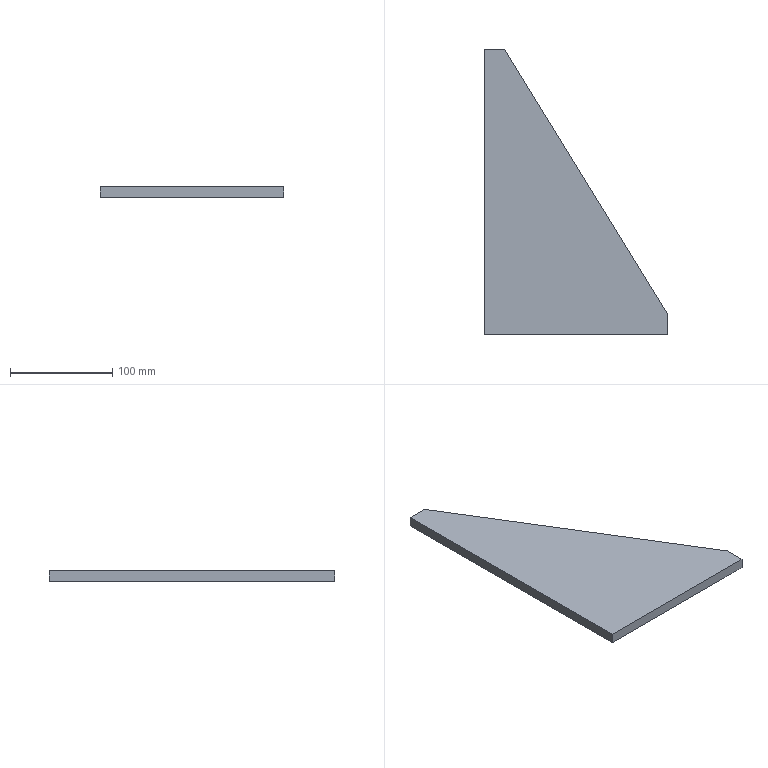Part | SolidWorks | features Extrusion 1 | 1 solid | 7 faces | box 180 x 280 x 10 mm | volume 296000 mm3 | plane 7
STEP:
#1=CARTESIAN_POINT('',(0.,0.,0.));
#2=VERTEX_POINT('',#1);
#3=CARTESIAN_POINT('',(180.,0.,0.));
#4=VERTEX_POINT('',#3);
#5=CARTESIAN_POINT('',(180.,0.,0.));
#6=DIRECTION('',(1.,0.,0.));
#7=VECTOR('',#6,1000.);
#8=LINE('',#5,#7);
#9=EDGE_CURVE('',#2,#4,#8,.T.);
#10=ORIENTED_EDGE('',*,*,#9,.T.);
#11=CARTESIAN_POINT('',(180.,0.,10.));
#12=VERTEX_POINT('',#11);
#13=CARTESIAN_POINT('',(180.,0.,10.));
#14=DIRECTION('',(0.,0.,-1.));
#15=VECTOR('',#14,1000.);
#16=LINE('',#13,#15);
#17=EDGE_CURVE('',#12,#4,#16,.T.);
#18=ORIENTED_EDGE('',*,*,#17,.F.);
#19=CARTESIAN_POINT('',(0.,0.,10.));
#20=VERTEX_POINT('',#19);
#21=CARTESIAN_POINT('',(180.,0.,10.));
#22=DIRECTION('',(1.,0.,0.));
#23=VECTOR('',#22,1000.);
#24=LINE('',#21,#23);
#25=EDGE_CURVE('',#20,#12,#24,.T.);
#26=ORIENTED_EDGE('',*,*,#25,.F.);
#27=CARTESIAN_POINT('',(0.,0.,10.));
#28=DIRECTION('',(0.,0.,-1.));
#29=VECTOR('',#28,1000.);
#30=LINE('',#27,#29);
#31=EDGE_CURVE('',#20,#2,#30,.T.);
#32=ORIENTED_EDGE('',*,*,#31,.T.);
#33=EDGE_LOOP('',(#10,#18,#26,#32));
#34=FACE_OUTER_BOUND('',#33,.T.);
#35=CARTESIAN_POINT('',(180.,0.,10.));
#36=DIRECTION('',(0.,1.,0.));
#37=DIRECTION('',(0.,0.,1.));
#38=AXIS2_PLACEMENT_3D('',#35,#36,#37);
#39=PLANE('',#38);
#40=ADVANCED_FACE('',(#34),#39,.F.);
#41=CARTESIAN_POINT('',(180.,20.,0.));
#42=VERTEX_POINT('',#41);
#43=CARTESIAN_POINT('',(180.,20.,0.));
#44=DIRECTION('',(0.,1.,0.));
#45=VECTOR('',#44,1000.);
#46=LINE('',#43,#45);
#47=EDGE_CURVE('',#4,#42,#46,.T.);
#48=ORIENTED_EDGE('',*,*,#47,.T.);
#49=CARTESIAN_POINT('',(180.,20.,10.));
#50=VERTEX_POINT('',#49);
#51=CARTESIAN_POINT('',(180.,20.,10.));
#52=DIRECTION('',(0.,0.,-1.));
#53=VECTOR('',#52,1000.);
#54=LINE('',#51,#53);
#55=EDGE_CURVE('',#50,#42,#54,.T.);
#56=ORIENTED_EDGE('',*,*,#55,.F.);
#57=CARTESIAN_POINT('',(180.,20.,10.));
#58=DIRECTION('',(0.,1.,0.));
#59=VECTOR('',#58,1000.);
#60=LINE('',#57,#59);
#61=EDGE_CURVE('',#12,#50,#60,.T.);
#62=ORIENTED_EDGE('',*,*,#61,.F.);
#63=ORIENTED_EDGE('',*,*,#17,.T.);
#64=EDGE_LOOP('',(#48,#56,#62,#63));
#65=FACE_OUTER_BOUND('',#64,.T.);
#66=CARTESIAN_POINT('',(180.,20.,10.));
#67=DIRECTION('',(-1.,0.,0.));
#68=DIRECTION('',(0.,0.,1.));
#69=AXIS2_PLACEMENT_3D('',#66,#67,#68);
#70=PLANE('',#69);
#71=ADVANCED_FACE('',(#65),#70,.F.);
#72=CARTESIAN_POINT('',(20.,280.,0.));
#73=VERTEX_POINT('',#72);
#74=CARTESIAN_POINT('',(20.,280.,0.));
#75=DIRECTION('',(-0.5241,0.8517,0.));
#76=VECTOR('',#75,1000.);
#77=LINE('',#74,#76);
#78=EDGE_CURVE('',#42,#73,#77,.T.);
#79=ORIENTED_EDGE('',*,*,#78,.T.);
#80=CARTESIAN_POINT('',(20.,280.,10.));
#81=VERTEX_POINT('',#80);
#82=CARTESIAN_POINT('',(20.,280.,10.));
#83=DIRECTION('',(0.,0.,-1.));
#84=VECTOR('',#83,1000.);
#85=LINE('',#82,#84);
#86=EDGE_CURVE('',#81,#73,#85,.T.);
#87=ORIENTED_EDGE('',*,*,#86,.F.);
#88=CARTESIAN_POINT('',(20.,280.,10.));
#89=DIRECTION('',(-0.5241,0.8517,0.));
#90=VECTOR('',#89,1000.);
#91=LINE('',#88,#90);
#92=EDGE_CURVE('',#50,#81,#91,.T.);
#93=ORIENTED_EDGE('',*,*,#92,.F.);
#94=ORIENTED_EDGE('',*,*,#55,.T.);
#95=EDGE_LOOP('',(#79,#87,#93,#94));
#96=FACE_OUTER_BOUND('',#95,.T.);
#97=CARTESIAN_POINT('',(20.,280.,10.));
#98=DIRECTION('',(-0.8517,-0.5241,0.));
#99=DIRECTION('',(0.5241,-0.8517,0.));
#100=AXIS2_PLACEMENT_3D('',#97,#98,#99);
#101=PLANE('',#100);
#102=ADVANCED_FACE('',(#96),#101,.F.);
#103=CARTESIAN_POINT('',(0.,280.,0.));
#104=VERTEX_POINT('',#103);
#105=CARTESIAN_POINT('',(0.,280.,0.));
#106=DIRECTION('',(-1.,0.,0.));
#107=VECTOR('',#106,1000.);
#108=LINE('',#105,#107);
#109=EDGE_CURVE('',#73,#104,#108,.T.);
#110=ORIENTED_EDGE('',*,*,#109,.T.);
#111=CARTESIAN_POINT('',(0.,280.,10.));
#112=VERTEX_POINT('',#111);
#113=CARTESIAN_POINT('',(0.,280.,10.));
#114=DIRECTION('',(0.,0.,-1.));
#115=VECTOR('',#114,1000.);
#116=LINE('',#113,#115);
#117=EDGE_CURVE('',#112,#104,#116,.T.);
#118=ORIENTED_EDGE('',*,*,#117,.F.);
#119=CARTESIAN_POINT('',(0.,280.,10.));
#120=DIRECTION('',(-1.,0.,0.));
#121=VECTOR('',#120,1000.);
#122=LINE('',#119,#121);
#123=EDGE_CURVE('',#81,#112,#122,.T.);
#124=ORIENTED_EDGE('',*,*,#123,.F.);
#125=ORIENTED_EDGE('',*,*,#86,.T.);
#126=EDGE_LOOP('',(#110,#118,#124,#125));
#127=FACE_OUTER_BOUND('',#126,.T.);
#128=CARTESIAN_POINT('',(0.,280.,10.));
#129=DIRECTION('',(0.,-1.,0.));
#130=DIRECTION('',(0.,0.,-1.));
#131=AXIS2_PLACEMENT_3D('',#128,#129,#130);
#132=PLANE('',#131);
#133=ADVANCED_FACE('',(#127),#132,.F.);
#134=CARTESIAN_POINT('',(0.,0.,0.));
#135=DIRECTION('',(0.,-1.,0.));
#136=VECTOR('',#135,1000.);
#137=LINE('',#134,#136);
#138=EDGE_CURVE('',#104,#2,#137,.T.);
#139=ORIENTED_EDGE('',*,*,#138,.T.);
#140=ORIENTED_EDGE('',*,*,#31,.F.);
#141=CARTESIAN_POINT('',(0.,0.,10.));
#142=DIRECTION('',(0.,-1.,0.));
#143=VECTOR('',#142,1000.);
#144=LINE('',#141,#143);
#145=EDGE_CURVE('',#112,#20,#144,.T.);
#146=ORIENTED_EDGE('',*,*,#145,.F.);
#147=ORIENTED_EDGE('',*,*,#117,.T.);
#148=EDGE_LOOP('',(#139,#140,#146,#147));
#149=FACE_OUTER_BOUND('',#148,.T.);
#150=CARTESIAN_POINT('',(0.,0.,10.));
#151=DIRECTION('',(1.,0.,0.));
#152=DIRECTION('',(0.,0.,-1.));
#153=AXIS2_PLACEMENT_3D('',#150,#151,#152);
#154=PLANE('',#153);
#155=ADVANCED_FACE('',(#149),#154,.F.);
#156=ORIENTED_EDGE('',*,*,#25,.T.);
#157=ORIENTED_EDGE('',*,*,#61,.T.);
#158=ORIENTED_EDGE('',*,*,#92,.T.);
#159=ORIENTED_EDGE('',*,*,#123,.T.);
#160=ORIENTED_EDGE('',*,*,#145,.T.);
#161=EDGE_LOOP('',(#156,#157,#158,#159,#160));
#162=FACE_OUTER_BOUND('',#161,.T.);
#163=CARTESIAN_POINT('',(0.,0.,10.));
#164=DIRECTION('',(0.,0.,-1.));
#165=DIRECTION('',(-1.,0.,0.));
#166=AXIS2_PLACEMENT_3D('',#163,#164,#165);
#167=PLANE('',#166);
#168=ADVANCED_FACE('',(#162),#167,.F.);
#169=ORIENTED_EDGE('',*,*,#9,.F.);
#170=ORIENTED_EDGE('',*,*,#138,.F.);
#171=ORIENTED_EDGE('',*,*,#109,.F.);
#172=ORIENTED_EDGE('',*,*,#78,.F.);
#173=ORIENTED_EDGE('',*,*,#47,.F.);
#174=EDGE_LOOP('',(#169,#170,#171,#172,#173));
#175=FACE_OUTER_BOUND('',#174,.T.);
#176=CARTESIAN_POINT('',(0.,0.,0.));
#177=DIRECTION('',(0.,0.,-1.));
#178=DIRECTION('',(-1.,0.,0.));
#179=AXIS2_PLACEMENT_3D('',#176,#177,#178);
#180=PLANE('',#179);
#181=ADVANCED_FACE('',(#175),#180,.T.);
#182=CLOSED_SHELL('',(#40,#71,#102,#133,#155,#168,#181));
#183=MANIFOLD_SOLID_BREP('',#182);
#184=CARTESIAN_POINT('',(0.,0.,0.));
#185=DIRECTION('',(0.,0.,1.));
#186=DIRECTION('',(1.,0.,0.));
#187=AXIS2_PLACEMENT_3D('',#184,#185,#186);
#188=(LENGTH_UNIT()NAMED_UNIT(*)SI_UNIT(.MILLI.,.METRE.));
#189=UNCERTAINTY_MEASURE_WITH_UNIT(LENGTH_MEASURE(0.00001),#188,'','');
#190=(NAMED_UNIT(*)PLANE_ANGLE_UNIT()SI_UNIT($,.RADIAN.));
#191=(NAMED_UNIT(*)SI_UNIT($,.STERADIAN.)SOLID_ANGLE_UNIT());
#192=(GEOMETRIC_REPRESENTATION_CONTEXT(3)GLOBAL_UNCERTAINTY_ASSIGNED_CONTEXT((#189))GLOBAL_UNIT_ASSIGNED_CONTEXT((#188,#190,#191))REPRESENTATION_CONTEXT('',''));
#193=ADVANCED_BREP_SHAPE_REPRESENTATION('',(#183,#187),#192);